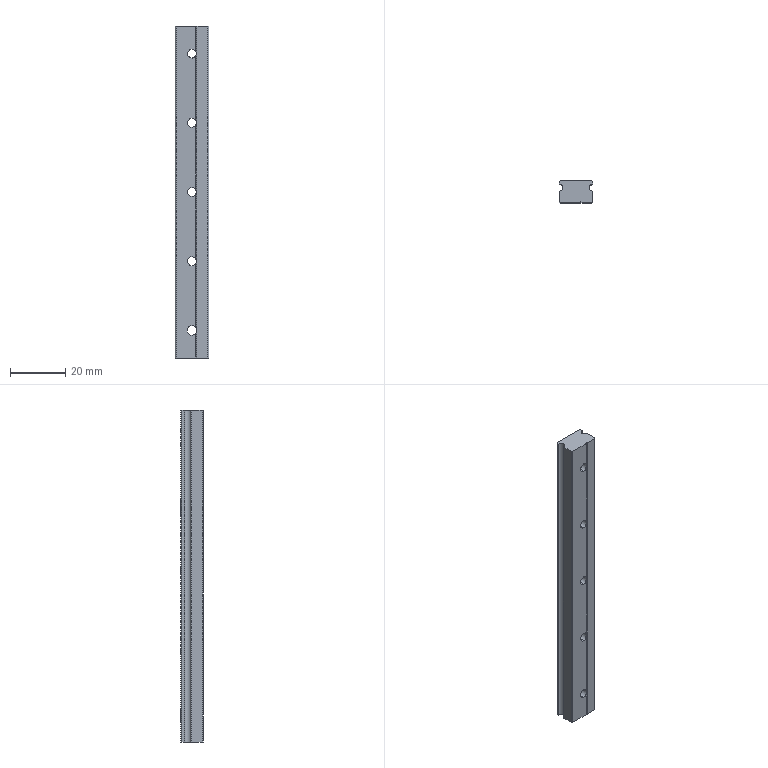Part | STEP file | Mount electronic clip MGN12C (slide rail) Z-axis | 1 solid | 42 faces | box 12 x 8 x 120 mm | volume 10218 mm3 | cylinder 24 | plane 18 | commonest cylinder face diameters 6 x10 3.2 x8 2.5 x3 3.5 x2 0.6 x1